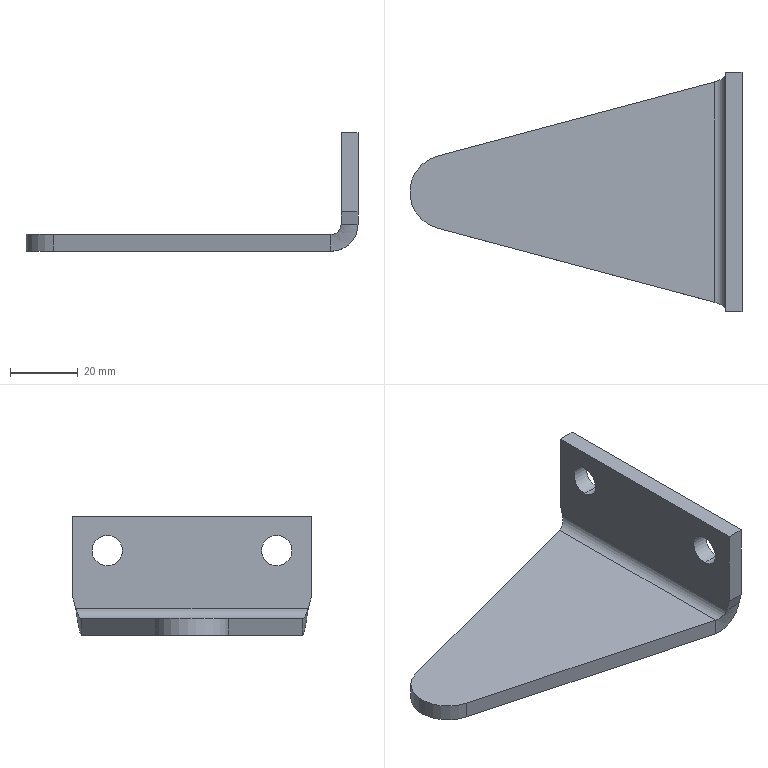Part | SolidWorks | features Fillet 2, BaseBody 1, HoleWzd 1, ICE 1 | 1 solid | 20 faces | box 97.999 x 70.526 x 35.001 mm | volume 30038 mm3 | plane 11 | cylinder 7 | spline 2 | commonest cylinder face diameters 9 x4 6 x1 16 x1 22 x1
STEP:
#1=CARTESIAN_POINT('',(-18.504,39.063,3.138));
#2=VERTEX_POINT('',#1);
#3=CARTESIAN_POINT('',(-18.504,39.063,2.784));
#4=VERTEX_POINT('',#3);
#5=CARTESIAN_POINT('',(-18.504,39.063,2.961));
#6=DIRECTION('',(1.,0.,0.));
#7=DIRECTION('',(0.,1.,0.));
#8=AXIS2_PLACEMENT_3D('',#5,#6,#7);
#9=CIRCLE('',#8,0.1772);
#10=EDGE_CURVE('',#2,#4,#9,.T.);
#11=ORIENTED_EDGE('',*,*,#10,.F.);
#12=CARTESIAN_POINT('',(-18.307,39.063,3.138));
#13=VERTEX_POINT('',#12);
#14=CARTESIAN_POINT('',(-18.307,39.063,3.138));
#15=DIRECTION('',(1.,0.,0.));
#16=VECTOR('',#15,39.37);
#17=LINE('',#14,#16);
#18=EDGE_CURVE('',#2,#13,#17,.T.);
#19=ORIENTED_EDGE('',*,*,#18,.T.);
#20=CARTESIAN_POINT('',(-18.307,39.063,2.784));
#21=VERTEX_POINT('',#20);
#22=CARTESIAN_POINT('',(-18.307,39.063,2.961));
#23=DIRECTION('',(1.,0.,0.));
#24=DIRECTION('',(0.,0.,-1.));
#25=AXIS2_PLACEMENT_3D('',#22,#23,#24);
#26=CIRCLE('',#25,0.1772);
#27=EDGE_CURVE('',#13,#21,#26,.T.);
#28=ORIENTED_EDGE('',*,*,#27,.T.);
#29=CARTESIAN_POINT('',(-18.307,39.063,2.784));
#30=DIRECTION('',(1.,0.,0.));
#31=VECTOR('',#30,39.37);
#32=LINE('',#29,#31);
#33=EDGE_CURVE('',#4,#21,#32,.T.);
#34=ORIENTED_EDGE('',*,*,#33,.F.);
#35=EDGE_LOOP('',(#11,#19,#28,#34));
#36=FACE_OUTER_BOUND('',#35,.T.);
#37=CARTESIAN_POINT('',(-18.307,39.063,2.961));
#38=DIRECTION('',(1.,0.,0.));
#39=DIRECTION('',(0.,0.,-1.));
#40=AXIS2_PLACEMENT_3D('',#37,#38,#39);
#41=CYLINDRICAL_SURFACE('',#40,0.1772);
#42=ADVANCED_FACE('',(#36),#41,.F.);
#43=CARTESIAN_POINT('',(-18.504,37.094,3.138));
#44=VERTEX_POINT('',#43);
#45=CARTESIAN_POINT('',(-18.504,37.094,2.784));
#46=VERTEX_POINT('',#45);
#47=CARTESIAN_POINT('',(-18.504,37.094,2.961));
#48=DIRECTION('',(1.,0.,0.));
#49=DIRECTION('',(0.,1.,0.));
#50=AXIS2_PLACEMENT_3D('',#47,#48,#49);
#51=CIRCLE('',#50,0.1772);
#52=EDGE_CURVE('',#44,#46,#51,.T.);
#53=ORIENTED_EDGE('',*,*,#52,.F.);
#54=CARTESIAN_POINT('',(-18.307,37.094,3.138));
#55=VERTEX_POINT('',#54);
#56=CARTESIAN_POINT('',(-18.307,37.094,3.138));
#57=DIRECTION('',(1.,0.,0.));
#58=VECTOR('',#57,39.37);
#59=LINE('',#56,#58);
#60=EDGE_CURVE('',#44,#55,#59,.T.);
#61=ORIENTED_EDGE('',*,*,#60,.T.);
#62=CARTESIAN_POINT('',(-18.307,37.094,2.784));
#63=VERTEX_POINT('',#62);
#64=CARTESIAN_POINT('',(-18.307,37.094,2.961));
#65=DIRECTION('',(1.,0.,0.));
#66=DIRECTION('',(0.,0.,-1.));
#67=AXIS2_PLACEMENT_3D('',#64,#65,#66);
#68=CIRCLE('',#67,0.1772);
#69=EDGE_CURVE('',#55,#63,#68,.T.);
#70=ORIENTED_EDGE('',*,*,#69,.T.);
#71=CARTESIAN_POINT('',(-18.307,37.094,2.784));
#72=DIRECTION('',(1.,0.,0.));
#73=VECTOR('',#72,39.37);
#74=LINE('',#71,#73);
#75=EDGE_CURVE('',#46,#63,#74,.T.);
#76=ORIENTED_EDGE('',*,*,#75,.F.);
#77=EDGE_LOOP('',(#53,#61,#70,#76));
#78=FACE_OUTER_BOUND('',#77,.T.);
#79=CARTESIAN_POINT('',(-18.307,37.094,2.961));
#80=DIRECTION('',(1.,0.,0.));
#81=DIRECTION('',(0.,0.,-1.));
#82=AXIS2_PLACEMENT_3D('',#79,#80,#81);
#83=CYLINDRICAL_SURFACE('',#82,0.1772);
#84=ADVANCED_FACE('',(#78),#83,.F.);
#85=CARTESIAN_POINT('',(-21.844,38.497,1.976));
#86=VERTEX_POINT('',#85);
#87=CARTESIAN_POINT('',(-18.622,39.358,1.976));
#88=VERTEX_POINT('',#87);
#89=CARTESIAN_POINT('',(-21.844,38.497,1.976));
#90=DIRECTION('',(0.9661,0.2581,0.));
#91=VECTOR('',#90,39.37);
#92=LINE('',#89,#91);
#93=EDGE_CURVE('',#86,#88,#92,.T.);
#94=ORIENTED_EDGE('',*,*,#93,.T.);
#95=CARTESIAN_POINT('',(-18.622,36.8,1.976));
#96=VERTEX_POINT('',#95);
#97=CARTESIAN_POINT('',(-18.622,38.079,1.976));
#98=DIRECTION('',(0.,-1.,0.));
#99=VECTOR('',#98,39.37);
#100=LINE('',#97,#99);
#101=EDGE_CURVE('',#88,#96,#100,.T.);
#102=ORIENTED_EDGE('',*,*,#101,.T.);
#103=CARTESIAN_POINT('',(-21.844,37.66,1.976));
#104=VERTEX_POINT('',#103);
#105=CARTESIAN_POINT('',(-18.622,36.8,1.976));
#106=DIRECTION('',(-0.9661,0.2581,0.));
#107=VECTOR('',#106,39.37);
#108=LINE('',#105,#107);
#109=EDGE_CURVE('',#96,#104,#108,.T.);
#110=ORIENTED_EDGE('',*,*,#109,.T.);
#111=CARTESIAN_POINT('',(-21.732,38.079,1.976));
#112=DIRECTION('',(0.,0.,-1.));
#113=DIRECTION('',(0.,1.,0.));
#114=AXIS2_PLACEMENT_3D('',#111,#112,#113);
#115=CIRCLE('',#114,0.4331);
#116=EDGE_CURVE('',#104,#86,#115,.T.);
#117=ORIENTED_EDGE('',*,*,#116,.T.);
#118=EDGE_LOOP('',(#94,#102,#110,#117));
#119=FACE_OUTER_BOUND('',#118,.T.);
#120=CARTESIAN_POINT('',(-21.732,38.079,1.976));
#121=DIRECTION('',(0.,0.,-1.));
#122=DIRECTION('',(0.,-1.,0.));
#123=AXIS2_PLACEMENT_3D('',#120,#121,#122);
#124=PLANE('',#123);
#125=ADVANCED_FACE('',(#119),#124,.T.);
#126=CARTESIAN_POINT('',(-21.844,38.497,2.173));
#127=VERTEX_POINT('',#126);
#128=CARTESIAN_POINT('',(-21.844,38.497,2.173));
#129=DIRECTION('',(0.,0.,1.));
#130=VECTOR('',#129,39.37);
#131=LINE('',#128,#130);
#132=EDGE_CURVE('',#86,#127,#131,.T.);
#133=ORIENTED_EDGE('',*,*,#132,.T.);
#134=CARTESIAN_POINT('',(-18.622,39.358,2.173));
#135=VERTEX_POINT('',#134);
#136=CARTESIAN_POINT('',(-21.844,38.497,2.173));
#137=DIRECTION('',(0.9661,0.2581,0.));
#138=VECTOR('',#137,39.37);
#139=LINE('',#136,#138);
#140=EDGE_CURVE('',#127,#135,#139,.T.);
#141=ORIENTED_EDGE('',*,*,#140,.T.);
#142=CARTESIAN_POINT('',(-18.622,39.358,2.173));
#143=DIRECTION('',(0.,0.,-1.));
#144=VECTOR('',#143,39.37);
#145=LINE('',#142,#144);
#146=EDGE_CURVE('',#135,#88,#145,.T.);
#147=ORIENTED_EDGE('',*,*,#146,.T.);
#148=ORIENTED_EDGE('',*,*,#93,.F.);
#149=EDGE_LOOP('',(#133,#141,#147,#148));
#150=FACE_OUTER_BOUND('',#149,.T.);
#151=CARTESIAN_POINT('',(-21.844,38.497,2.173));
#152=DIRECTION('',(-0.2581,0.9661,0.));
#153=DIRECTION('',(0.9661,0.2581,0.));
#154=AXIS2_PLACEMENT_3D('',#151,#152,#153);
#155=PLANE('',#154);
#156=ADVANCED_FACE('',(#150),#155,.T.);
#157=CARTESIAN_POINT('',(-21.844,37.66,2.173));
#158=VERTEX_POINT('',#157);
#159=CARTESIAN_POINT('',(-21.732,38.079,2.173));
#160=DIRECTION('',(0.,0.,-1.));
#161=DIRECTION('',(0.,1.,0.));
#162=AXIS2_PLACEMENT_3D('',#159,#160,#161);
#163=CIRCLE('',#162,0.4331);
#164=EDGE_CURVE('',#158,#127,#163,.T.);
#165=ORIENTED_EDGE('',*,*,#164,.T.);
#166=ORIENTED_EDGE('',*,*,#132,.F.);
#167=ORIENTED_EDGE('',*,*,#116,.F.);
#168=CARTESIAN_POINT('',(-21.844,37.66,2.173));
#169=DIRECTION('',(0.,0.,1.));
#170=VECTOR('',#169,39.37);
#171=LINE('',#168,#170);
#172=EDGE_CURVE('',#104,#158,#171,.T.);
#173=ORIENTED_EDGE('',*,*,#172,.T.);
#174=EDGE_LOOP('',(#165,#166,#167,#173));
#175=FACE_OUTER_BOUND('',#174,.T.);
#176=CARTESIAN_POINT('',(-21.732,38.079,2.173));
#177=DIRECTION('',(0.,0.,1.));
#178=DIRECTION('',(0.,1.,0.));
#179=AXIS2_PLACEMENT_3D('',#176,#177,#178);
#180=CYLINDRICAL_SURFACE('',#179,0.4331);
#181=ADVANCED_FACE('',(#175),#180,.T.);
#182=CARTESIAN_POINT('',(-18.622,36.8,2.173));
#183=VERTEX_POINT('',#182);
#184=CARTESIAN_POINT('',(-18.031,36.642,2.173));
#185=DIRECTION('',(-0.9661,0.2581,0.));
#186=VECTOR('',#185,39.37);
#187=LINE('',#184,#186);
#188=EDGE_CURVE('',#183,#158,#187,.T.);
#189=ORIENTED_EDGE('',*,*,#188,.T.);
#190=ORIENTED_EDGE('',*,*,#172,.F.);
#191=ORIENTED_EDGE('',*,*,#109,.F.);
#192=CARTESIAN_POINT('',(-18.622,36.8,2.173));
#193=DIRECTION('',(0.,0.,1.));
#194=VECTOR('',#193,39.37);
#195=LINE('',#192,#194);
#196=EDGE_CURVE('',#96,#183,#195,.T.);
#197=ORIENTED_EDGE('',*,*,#196,.T.);
#198=EDGE_LOOP('',(#189,#190,#191,#197));
#199=FACE_OUTER_BOUND('',#198,.T.);
#200=CARTESIAN_POINT('',(-18.031,36.642,2.173));
#201=DIRECTION('',(-0.2581,-0.9661,0.));
#202=DIRECTION('',(-0.9661,0.2581,0.));
#203=AXIS2_PLACEMENT_3D('',#200,#201,#202);
#204=PLANE('',#203);
#205=ADVANCED_FACE('',(#199),#204,.T.);
#206=ORIENTED_EDGE('',*,*,#188,.F.);
#207=CARTESIAN_POINT('',(-18.622,39.393,2.173));
#208=DIRECTION('',(0.,1.,0.));
#209=VECTOR('',#208,39.37);
#210=LINE('',#207,#209);
#211=EDGE_CURVE('',#183,#135,#210,.T.);
#212=ORIENTED_EDGE('',*,*,#211,.T.);
#213=ORIENTED_EDGE('',*,*,#140,.F.);
#214=ORIENTED_EDGE('',*,*,#164,.F.);
#215=EDGE_LOOP('',(#206,#212,#213,#214));
#216=FACE_OUTER_BOUND('',#215,.T.);
#217=CARTESIAN_POINT('',(-21.732,38.079,2.173));
#218=DIRECTION('',(0.,0.,-1.));
#219=DIRECTION('',(0.,-1.,0.));
#220=AXIS2_PLACEMENT_3D('',#217,#218,#219);
#221=PLANE('',#220);
#222=ADVANCED_FACE('',(#216),#221,.F.);
#223=CARTESIAN_POINT('',(-18.307,39.429,2.291));
#224=VERTEX_POINT('',#223);
#225=CARTESIAN_POINT('',(-18.504,39.429,2.291));
#226=VERTEX_POINT('',#225);
#227=CARTESIAN_POINT('',(-18.406,39.429,2.291));
#228=DIRECTION('',(-1.,0.,0.));
#229=VECTOR('',#228,39.37);
#230=LINE('',#227,#229);
#231=EDGE_CURVE('',#224,#226,#230,.T.);
#232=ORIENTED_EDGE('',*,*,#231,.F.);
#233=CARTESIAN_POINT('',(-18.307,39.429,2.291));
#234=CARTESIAN_POINT('',(-18.307,39.426,2.271));
#235=CARTESIAN_POINT('',(-18.309,39.423,2.25));
#236=CARTESIAN_POINT('',(-18.315,39.419,2.22));
#237=CARTESIAN_POINT('',(-18.318,39.417,2.21));
#238=CARTESIAN_POINT('',(-18.324,39.414,2.19));
#239=CARTESIAN_POINT('',(-18.327,39.413,2.18));
#240=CARTESIAN_POINT('',(-18.339,39.408,2.152));
#241=CARTESIAN_POINT('',(-18.349,39.405,2.134));
#242=CARTESIAN_POINT('',(-18.371,39.399,2.1));
#243=CARTESIAN_POINT('',(-18.385,39.396,2.083));
#244=CARTESIAN_POINT('',(-18.414,39.39,2.054));
#245=CARTESIAN_POINT('',(-18.43,39.388,2.041));
#246=CARTESIAN_POINT('',(-18.455,39.383,2.024));
#247=CARTESIAN_POINT('',(-18.464,39.382,2.019));
#248=CARTESIAN_POINT('',(-18.483,39.379,2.009));
#249=CARTESIAN_POINT('',(-18.492,39.377,2.004));
#250=CARTESIAN_POINT('',(-18.52,39.373,1.993));
#251=CARTESIAN_POINT('',(-18.54,39.37,1.987));
#252=CARTESIAN_POINT('',(-18.581,39.364,1.978));
#253=CARTESIAN_POINT('',(-18.601,39.361,1.976));
#254=CARTESIAN_POINT('',(-18.622,39.358,1.976));
#255=B_SPLINE_CURVE_WITH_KNOTS('',3,(#233,#234,#235,#236,#237,#238,#239,#240,#241,#242,#243,#244,#245,#246,#247,#248,#249,#250,#251,#252,#253,#254),.UNSPECIFIED.,.F.,.F.,(4,2,2,2,2,2,2,2,2,2,4),(0.,0.001578,0.002367,0.003156,0.004734,0.006312,0.00789,0.008679,0.009468,0.01105,0.01262),.UNSPECIFIED.);
#256=EDGE_CURVE('',#224,#88,#255,.T.);
#257=ORIENTED_EDGE('',*,*,#256,.T.);
#258=ORIENTED_EDGE('',*,*,#146,.F.);
#259=CARTESIAN_POINT('',(-18.622,39.358,2.173));
#260=CARTESIAN_POINT('',(-18.614,39.361,2.173));
#261=CARTESIAN_POINT('',(-18.607,39.364,2.174));
#262=CARTESIAN_POINT('',(-18.591,39.37,2.177));
#263=CARTESIAN_POINT('',(-18.584,39.373,2.179));
#264=CARTESIAN_POINT('',(-18.57,39.379,2.185));
#265=CARTESIAN_POINT('',(-18.563,39.382,2.189));
#266=CARTESIAN_POINT('',(-18.55,39.387,2.197));
#267=CARTESIAN_POINT('',(-18.544,39.39,2.202));
#268=CARTESIAN_POINT('',(-18.533,39.396,2.213));
#269=CARTESIAN_POINT('',(-18.528,39.399,2.219));
#270=CARTESIAN_POINT('',(-18.52,39.405,2.232));
#271=CARTESIAN_POINT('',(-18.516,39.408,2.239));
#272=CARTESIAN_POINT('',(-18.51,39.414,2.253));
#273=CARTESIAN_POINT('',(-18.508,39.417,2.261));
#274=CARTESIAN_POINT('',(-18.505,39.423,2.276));
#275=CARTESIAN_POINT('',(-18.504,39.426,2.284));
#276=CARTESIAN_POINT('',(-18.504,39.429,2.291));
#277=B_SPLINE_CURVE_WITH_KNOTS('',3,(#259,#260,#261,#262,#263,#264,#265,#266,#267,#268,#269,#270,#271,#272,#273,#274,#275,#276),.UNSPECIFIED.,.F.,.F.,(4,2,2,2,2,2,2,2,4),(0.,0.0006272,0.001254,0.001881,0.002509,0.003136,0.003763,0.00439,0.005017),.UNSPECIFIED.);
#278=EDGE_CURVE('',#135,#226,#277,.T.);
#279=ORIENTED_EDGE('',*,*,#278,.T.);
#280=EDGE_LOOP('',(#232,#257,#258,#279));
#281=FACE_OUTER_BOUND('',#280,.T.);
#282=CARTESIAN_POINT('',(-18.175,39.429,2.291));
#283=CARTESIAN_POINT('',(-18.175,39.423,2.233));
#284=CARTESIAN_POINT('',(-18.186,39.417,2.174));
#285=CARTESIAN_POINT('',(-18.231,39.405,2.066));
#286=CARTESIAN_POINT('',(-18.264,39.399,2.016));
#287=CARTESIAN_POINT('',(-18.347,39.387,1.934));
#288=CARTESIAN_POINT('',(-18.397,39.382,1.9));
#289=CARTESIAN_POINT('',(-18.505,39.37,1.856));
#290=CARTESIAN_POINT('',(-18.563,39.364,1.844));
#291=CARTESIAN_POINT('',(-18.622,39.358,1.844));
#292=CARTESIAN_POINT('',(-18.305,39.429,2.291));
#293=CARTESIAN_POINT('',(-18.305,39.423,2.25));
#294=CARTESIAN_POINT('',(-18.313,39.417,2.208));
#295=CARTESIAN_POINT('',(-18.345,39.405,2.132));
#296=CARTESIAN_POINT('',(-18.369,39.399,2.097));
#297=CARTESIAN_POINT('',(-18.427,39.387,2.038));
#298=CARTESIAN_POINT('',(-18.462,39.382,2.014));
#299=CARTESIAN_POINT('',(-18.539,39.37,1.983));
#300=CARTESIAN_POINT('',(-18.581,39.364,1.974));
#301=CARTESIAN_POINT('',(-18.622,39.358,1.974));
#302=CARTESIAN_POINT('',(-18.307,39.429,2.291));
#303=CARTESIAN_POINT('',(-18.307,39.423,2.25));
#304=CARTESIAN_POINT('',(-18.315,39.417,2.209));
#305=CARTESIAN_POINT('',(-18.347,39.405,2.133));
#306=CARTESIAN_POINT('',(-18.37,39.399,2.098));
#307=CARTESIAN_POINT('',(-18.428,39.387,2.04));
#308=CARTESIAN_POINT('',(-18.463,39.382,2.016));
#309=CARTESIAN_POINT('',(-18.54,39.37,1.985));
#310=CARTESIAN_POINT('',(-18.581,39.364,1.976));
#311=CARTESIAN_POINT('',(-18.622,39.358,1.976));
#312=CARTESIAN_POINT('',(-18.504,39.429,2.291));
#313=CARTESIAN_POINT('',(-18.504,39.423,2.276));
#314=CARTESIAN_POINT('',(-18.507,39.417,2.26));
#315=CARTESIAN_POINT('',(-18.519,39.405,2.232));
#316=CARTESIAN_POINT('',(-18.528,39.399,2.219));
#317=CARTESIAN_POINT('',(-18.549,39.387,2.197));
#318=CARTESIAN_POINT('',(-18.563,39.382,2.188));
#319=CARTESIAN_POINT('',(-18.591,39.37,2.176));
#320=CARTESIAN_POINT('',(-18.607,39.364,2.173));
#321=CARTESIAN_POINT('',(-18.622,39.358,2.173));
#322=CARTESIAN_POINT('',(-18.506,39.429,2.291));
#323=CARTESIAN_POINT('',(-18.506,39.423,2.276));
#324=CARTESIAN_POINT('',(-18.509,39.417,2.261));
#325=CARTESIAN_POINT('',(-18.521,39.405,2.233));
#326=CARTESIAN_POINT('',(-18.529,39.399,2.22));
#327=CARTESIAN_POINT('',(-18.551,39.387,2.199));
#328=CARTESIAN_POINT('',(-18.564,39.382,2.19));
#329=CARTESIAN_POINT('',(-18.592,39.37,2.178));
#330=CARTESIAN_POINT('',(-18.607,39.364,2.175));
#331=CARTESIAN_POINT('',(-18.622,39.358,2.175));
#332=B_SPLINE_SURFACE_WITH_KNOTS('',1,3,((#282,#283,#284,#285,#286,#287,#288,#289,#290,#291),(#292,#293,#294,#295,#296,#297,#298,#299,#300,#301),(#302,#303,#304,#305,#306,#307,#308,#309,#310,#311),(#312,#313,#314,#315,#316,#317,#318,#319,#320,#321),(#322,#323,#324,#325,#326,#327,#328,#329,#330,#331)),.UNSPECIFIED.,.F.,.F.,.F.,(2,1,1,1,2),(4,2,2,2,4),(-0.6727,-0.01,0.,1.,1.01),(0.,0.25,0.5,0.75,1.),.UNSPECIFIED.);
#333=ADVANCED_FACE('',(#281),#332,.F.);
#334=ORIENTED_EDGE('',*,*,#196,.F.);
#335=CARTESIAN_POINT('',(-18.307,36.729,2.291));
#336=VERTEX_POINT('',#335);
#337=CARTESIAN_POINT('',(-18.622,36.8,1.976));
#338=CARTESIAN_POINT('',(-18.601,36.797,1.976));
#339=CARTESIAN_POINT('',(-18.581,36.794,1.978));
#340=CARTESIAN_POINT('',(-18.551,36.789,1.984));
#341=CARTESIAN_POINT('',(-18.541,36.788,1.987));
#342=CARTESIAN_POINT('',(-18.521,36.785,1.993));
#343=CARTESIAN_POINT('',(-18.511,36.783,1.996));
#344=CARTESIAN_POINT('',(-18.482,36.779,2.008));
#345=CARTESIAN_POINT('',(-18.464,36.776,2.018));
#346=CARTESIAN_POINT('',(-18.43,36.77,2.041));
#347=CARTESIAN_POINT('',(-18.414,36.767,2.054));
#348=CARTESIAN_POINT('',(-18.385,36.761,2.083));
#349=CARTESIAN_POINT('',(-18.372,36.758,2.099));
#350=CARTESIAN_POINT('',(-18.355,36.754,2.125));
#351=CARTESIAN_POINT('',(-18.349,36.752,2.134));
#352=CARTESIAN_POINT('',(-18.339,36.749,2.152));
#353=CARTESIAN_POINT('',(-18.335,36.748,2.161));
#354=CARTESIAN_POINT('',(-18.323,36.743,2.19));
#355=CARTESIAN_POINT('',(-18.317,36.741,2.209));
#356=CARTESIAN_POINT('',(-18.309,36.735,2.25));
#357=CARTESIAN_POINT('',(-18.307,36.732,2.271));
#358=CARTESIAN_POINT('',(-18.307,36.729,2.291));
#359=B_SPLINE_CURVE_WITH_KNOTS('',3,(#337,#338,#339,#340,#341,#342,#343,#344,#345,#346,#347,#348,#349,#350,#351,#352,#353,#354,#355,#356,#357,#358),.UNSPECIFIED.,.F.,.F.,(4,2,2,2,2,2,2,2,2,2,4),(0.,0.001578,0.002367,0.003156,0.004734,0.006312,0.00789,0.008679,0.009468,0.01105,0.01262),.UNSPECIFIED.);
#360=EDGE_CURVE('',#96,#336,#359,.T.);
#361=ORIENTED_EDGE('',*,*,#360,.T.);
#362=CARTESIAN_POINT('',(-18.504,36.729,2.291));
#363=VERTEX_POINT('',#362);
#364=CARTESIAN_POINT('',(-18.406,36.729,2.291));
#365=DIRECTION('',(1.,0.,0.));
#366=VECTOR('',#365,39.37);
#367=LINE('',#364,#366);
#368=EDGE_CURVE('',#363,#336,#367,.T.);
#369=ORIENTED_EDGE('',*,*,#368,.F.);
#370=CARTESIAN_POINT('',(-18.504,36.729,2.291));
#371=CARTESIAN_POINT('',(-18.504,36.732,2.284));
#372=CARTESIAN_POINT('',(-18.505,36.735,2.276));
#373=CARTESIAN_POINT('',(-18.508,36.74,2.261));
#374=CARTESIAN_POINT('',(-18.51,36.743,2.253));
#375=CARTESIAN_POINT('',(-18.516,36.749,2.239));
#376=CARTESIAN_POINT('',(-18.52,36.752,2.232));
#377=CARTESIAN_POINT('',(-18.528,36.758,2.219));
#378=CARTESIAN_POINT('',(-18.533,36.761,2.213));
#379=CARTESIAN_POINT('',(-18.544,36.767,2.202));
#380=CARTESIAN_POINT('',(-18.55,36.77,2.198));
#381=CARTESIAN_POINT('',(-18.563,36.776,2.189));
#382=CARTESIAN_POINT('',(-18.57,36.779,2.185));
#383=CARTESIAN_POINT('',(-18.584,36.785,2.179));
#384=CARTESIAN_POINT('',(-18.591,36.788,2.177));
#385=CARTESIAN_POINT('',(-18.606,36.794,2.174));
#386=CARTESIAN_POINT('',(-18.614,36.797,2.173));
#387=CARTESIAN_POINT('',(-18.622,36.8,2.173));
#388=B_SPLINE_CURVE_WITH_KNOTS('',3,(#370,#371,#372,#373,#374,#375,#376,#377,#378,#379,#380,#381,#382,#383,#384,#385,#386,#387),.UNSPECIFIED.,.F.,.F.,(4,2,2,2,2,2,2,2,4),(0.,0.0006272,0.001254,0.001881,0.002509,0.003136,0.003763,0.00439,0.005017),.UNSPECIFIED.);
#389=EDGE_CURVE('',#363,#183,#388,.T.);
#390=ORIENTED_EDGE('',*,*,#389,.T.);
#391=EDGE_LOOP('',(#334,#361,#369,#390));
#392=FACE_OUTER_BOUND('',#391,.T.);
#393=CARTESIAN_POINT('',(-18.622,36.8,1.844));
#394=CARTESIAN_POINT('',(-18.563,36.794,1.844));
#395=CARTESIAN_POINT('',(-18.505,36.788,1.856));
#396=CARTESIAN_POINT('',(-18.397,36.776,1.9));
#397=CARTESIAN_POINT('',(-18.347,36.77,1.934));
#398=CARTESIAN_POINT('',(-18.264,36.758,2.016));
#399=CARTESIAN_POINT('',(-18.231,36.752,2.066));
#400=CARTESIAN_POINT('',(-18.186,36.74,2.174));
#401=CARTESIAN_POINT('',(-18.175,36.735,2.233));
#402=CARTESIAN_POINT('',(-18.175,36.729,2.291));
#403=CARTESIAN_POINT('',(-18.622,36.8,1.974));
#404=CARTESIAN_POINT('',(-18.581,36.794,1.974));
#405=CARTESIAN_POINT('',(-18.539,36.788,1.983));
#406=CARTESIAN_POINT('',(-18.462,36.776,2.014));
#407=CARTESIAN_POINT('',(-18.427,36.77,2.038));
#408=CARTESIAN_POINT('',(-18.369,36.758,2.097));
#409=CARTESIAN_POINT('',(-18.345,36.752,2.132));
#410=CARTESIAN_POINT('',(-18.313,36.74,2.208));
#411=CARTESIAN_POINT('',(-18.305,36.735,2.25));
#412=CARTESIAN_POINT('',(-18.305,36.729,2.291));
#413=CARTESIAN_POINT('',(-18.622,36.8,1.976));
#414=CARTESIAN_POINT('',(-18.581,36.794,1.976));
#415=CARTESIAN_POINT('',(-18.54,36.788,1.985));
#416=CARTESIAN_POINT('',(-18.463,36.776,2.016));
#417=CARTESIAN_POINT('',(-18.428,36.77,2.04));
#418=CARTESIAN_POINT('',(-18.37,36.758,2.098));
#419=CARTESIAN_POINT('',(-18.347,36.752,2.133));
#420=CARTESIAN_POINT('',(-18.315,36.74,2.209));
#421=CARTESIAN_POINT('',(-18.307,36.735,2.25));
#422=CARTESIAN_POINT('',(-18.307,36.729,2.291));
#423=CARTESIAN_POINT('',(-18.622,36.8,2.173));
#424=CARTESIAN_POINT('',(-18.607,36.794,2.173));
#425=CARTESIAN_POINT('',(-18.591,36.788,2.176));
#426=CARTESIAN_POINT('',(-18.563,36.776,2.188));
#427=CARTESIAN_POINT('',(-18.549,36.77,2.197));
#428=CARTESIAN_POINT('',(-18.528,36.758,2.219));
#429=CARTESIAN_POINT('',(-18.519,36.752,2.232));
#430=CARTESIAN_POINT('',(-18.507,36.74,2.26));
#431=CARTESIAN_POINT('',(-18.504,36.735,2.276));
#432=CARTESIAN_POINT('',(-18.504,36.729,2.291));
#433=CARTESIAN_POINT('',(-18.622,36.8,2.175));
#434=CARTESIAN_POINT('',(-18.607,36.794,2.175));
#435=CARTESIAN_POINT('',(-18.592,36.788,2.178));
#436=CARTESIAN_POINT('',(-18.564,36.776,2.19));
#437=CARTESIAN_POINT('',(-18.551,36.77,2.199));
#438=CARTESIAN_POINT('',(-18.529,36.758,2.22));
#439=CARTESIAN_POINT('',(-18.521,36.752,2.233));
#440=CARTESIAN_POINT('',(-18.509,36.74,2.261));
#441=CARTESIAN_POINT('',(-18.506,36.735,2.276));
#442=CARTESIAN_POINT('',(-18.506,36.729,2.291));
#443=B_SPLINE_SURFACE_WITH_KNOTS('',1,3,((#393,#394,#395,#396,#397,#398,#399,#400,#401,#402),(#403,#404,#405,#406,#407,#408,#409,#410,#411,#412),(#413,#414,#415,#416,#417,#418,#419,#420,#421,#422),(#423,#424,#425,#426,#427,#428,#429,#430,#431,#432),(#433,#434,#435,#436,#437,#438,#439,#440,#441,#442)),.UNSPECIFIED.,.F.,.F.,.F.,(2,1,1,1,2),(4,2,2,2,4),(-0.6727,-0.01,0.,1.,1.01),(0.,0.25,0.5,0.75,1.),.UNSPECIFIED.);
#444=ADVANCED_FACE('',(#392),#443,.F.);
#445=CARTESIAN_POINT('',(-18.307,39.063,2.961));
#446=DIRECTION('',(1.,0.,0.));
#447=DIRECTION('',(0.,0.,-1.));
#448=AXIS2_PLACEMENT_3D('',#445,#446,#447);
#449=CIRCLE('',#448,0.1772);
#450=EDGE_CURVE('',#21,#13,#449,.T.);
#451=ORIENTED_EDGE('',*,*,#450,.F.);
#452=ORIENTED_EDGE('',*,*,#27,.F.);
#453=EDGE_LOOP('',(#451,#452));
#454=FACE_BOUND('',#453,.T.);
#455=CARTESIAN_POINT('',(-18.307,37.094,2.961));
#456=DIRECTION('',(1.,0.,0.));
#457=DIRECTION('',(0.,0.,-1.));
#458=AXIS2_PLACEMENT_3D('',#455,#456,#457);
#459=CIRCLE('',#458,0.1772);
#460=EDGE_CURVE('',#63,#55,#459,.T.);
#461=ORIENTED_EDGE('',*,*,#460,.F.);
#462=ORIENTED_EDGE('',*,*,#69,.F.);
#463=EDGE_LOOP('',(#461,#462));
#464=FACE_BOUND('',#463,.T.);
#465=CARTESIAN_POINT('',(-18.307,36.69,2.434));
#466=VERTEX_POINT('',#465);
#467=CARTESIAN_POINT('',(-18.307,36.726,2.302));
#468=DIRECTION('',(0.,0.2581,-0.9661));
#469=VECTOR('',#468,39.37);
#470=LINE('',#467,#469);
#471=EDGE_CURVE('',#466,#336,#470,.T.);
#472=ORIENTED_EDGE('',*,*,#471,.T.);
#473=CARTESIAN_POINT('',(-18.307,38.079,2.291));
#474=DIRECTION('',(0.,1.,0.));
#475=VECTOR('',#474,39.37);
#476=LINE('',#473,#475);
#477=EDGE_CURVE('',#336,#224,#476,.T.);
#478=ORIENTED_EDGE('',*,*,#477,.T.);
#479=CARTESIAN_POINT('',(-18.307,39.467,2.434));
#480=VERTEX_POINT('',#479);
#481=CARTESIAN_POINT('',(-18.307,39.429,2.291));
#482=DIRECTION('',(0.,0.2581,0.9661));
#483=VECTOR('',#482,39.37);
#484=LINE('',#481,#483);
#485=EDGE_CURVE('',#224,#480,#484,.T.);
#486=ORIENTED_EDGE('',*,*,#485,.T.);
#487=CARTESIAN_POINT('',(-18.307,39.467,3.354));
#488=VERTEX_POINT('',#487);
#489=CARTESIAN_POINT('',(-18.307,39.467,3.354));
#490=DIRECTION('',(0.,0.,-1.));
#491=VECTOR('',#490,39.37);
#492=LINE('',#489,#491);
#493=EDGE_CURVE('',#488,#480,#492,.T.);
#494=ORIENTED_EDGE('',*,*,#493,.F.);
#495=CARTESIAN_POINT('',(-18.307,36.69,3.354));
#496=VERTEX_POINT('',#495);
#497=CARTESIAN_POINT('',(-18.307,39.467,3.354));
#498=DIRECTION('',(0.,1.,0.));
#499=VECTOR('',#498,39.37);
#500=LINE('',#497,#499);
#501=EDGE_CURVE('',#496,#488,#500,.T.);
#502=ORIENTED_EDGE('',*,*,#501,.F.);
#503=CARTESIAN_POINT('',(-18.307,36.69,3.354));
#504=DIRECTION('',(0.,0.,-1.));
#505=VECTOR('',#504,39.37);
#506=LINE('',#503,#505);
#507=EDGE_CURVE('',#496,#466,#506,.T.);
#508=ORIENTED_EDGE('',*,*,#507,.T.);
#509=EDGE_LOOP('',(#472,#478,#486,#494,#502,#508));
#510=FACE_OUTER_BOUND('',#509,.T.);
#511=CARTESIAN_POINT('',(-18.307,38.079,-1.084));
#512=DIRECTION('',(1.,0.,0.));
#513=DIRECTION('',(0.,0.,1.));
#514=AXIS2_PLACEMENT_3D('',#511,#512,#513);
#515=PLANE('',#514);
#516=ADVANCED_FACE('',(#454,#464,#510),#515,.T.);
#517=CARTESIAN_POINT('',(-18.504,39.467,2.434));
#518=VERTEX_POINT('',#517);
#519=CARTESIAN_POINT('',(-18.504,38.497,-1.196));
#520=DIRECTION('',(0.,0.2581,0.9661));
#521=VECTOR('',#520,39.37);
#522=LINE('',#519,#521);
#523=EDGE_CURVE('',#226,#518,#522,.T.);
#524=ORIENTED_EDGE('',*,*,#523,.T.);
#525=CARTESIAN_POINT('',(-18.504,39.467,2.434));
#526=DIRECTION('',(-1.,0.,0.));
#527=VECTOR('',#526,39.37);
#528=LINE('',#525,#527);
#529=EDGE_CURVE('',#480,#518,#528,.T.);
#530=ORIENTED_EDGE('',*,*,#529,.F.);
#531=ORIENTED_EDGE('',*,*,#485,.F.);
#532=ORIENTED_EDGE('',*,*,#231,.T.);
#533=EDGE_LOOP('',(#524,#530,#531,#532));
#534=FACE_OUTER_BOUND('',#533,.T.);
#535=CARTESIAN_POINT('',(-18.504,38.497,-1.196));
#536=DIRECTION('',(0.,0.9661,-0.2581));
#537=DIRECTION('',(0.,-0.2581,-0.9661));
#538=AXIS2_PLACEMENT_3D('',#535,#536,#537);
#539=PLANE('',#538);
#540=ADVANCED_FACE('',(#534),#539,.T.);
#541=ORIENTED_EDGE('',*,*,#471,.F.);
#542=CARTESIAN_POINT('',(-18.504,36.69,2.434));
#543=VERTEX_POINT('',#542);
#544=CARTESIAN_POINT('',(-18.504,36.69,2.434));
#545=DIRECTION('',(1.,0.,0.));
#546=VECTOR('',#545,39.37);
#547=LINE('',#544,#546);
#548=EDGE_CURVE('',#543,#466,#547,.T.);
#549=ORIENTED_EDGE('',*,*,#548,.F.);
#550=CARTESIAN_POINT('',(-18.504,36.642,2.617));
#551=DIRECTION('',(0.,0.2581,-0.9661));
#552=VECTOR('',#551,39.37);
#553=LINE('',#550,#552);
#554=EDGE_CURVE('',#543,#363,#553,.T.);
#555=ORIENTED_EDGE('',*,*,#554,.T.);
#556=ORIENTED_EDGE('',*,*,#368,.T.);
#557=EDGE_LOOP('',(#541,#549,#555,#556));
#558=FACE_OUTER_BOUND('',#557,.T.);
#559=CARTESIAN_POINT('',(-18.504,36.642,2.617));
#560=DIRECTION('',(0.,-0.9661,-0.2581));
#561=DIRECTION('',(0.,-0.2581,0.9661));
#562=AXIS2_PLACEMENT_3D('',#559,#560,#561);
#563=PLANE('',#562);
#564=ADVANCED_FACE('',(#558),#563,.T.);
#565=CARTESIAN_POINT('',(-18.504,39.063,2.961));
#566=DIRECTION('',(1.,0.,0.));
#567=DIRECTION('',(0.,1.,0.));
#568=AXIS2_PLACEMENT_3D('',#565,#566,#567);
#569=CIRCLE('',#568,0.1772);
#570=EDGE_CURVE('',#4,#2,#569,.T.);
#571=ORIENTED_EDGE('',*,*,#570,.T.);
#572=ORIENTED_EDGE('',*,*,#10,.T.);
#573=EDGE_LOOP('',(#571,#572));
#574=FACE_BOUND('',#573,.T.);
#575=CARTESIAN_POINT('',(-18.504,37.094,2.961));
#576=DIRECTION('',(1.,0.,0.));
#577=DIRECTION('',(0.,1.,0.));
#578=AXIS2_PLACEMENT_3D('',#575,#576,#577);
#579=CIRCLE('',#578,0.1772);
#580=EDGE_CURVE('',#46,#44,#579,.T.);
#581=ORIENTED_EDGE('',*,*,#580,.T.);
#582=ORIENTED_EDGE('',*,*,#52,.T.);
#583=EDGE_LOOP('',(#581,#582));
#584=FACE_BOUND('',#583,.T.);
#585=ORIENTED_EDGE('',*,*,#523,.F.);
#586=CARTESIAN_POINT('',(-18.504,36.764,2.291));
#587=DIRECTION('',(0.,-1.,0.));
#588=VECTOR('',#587,39.37);
#589=LINE('',#586,#588);
#590=EDGE_CURVE('',#226,#363,#589,.T.);
#591=ORIENTED_EDGE('',*,*,#590,.T.);
#592=ORIENTED_EDGE('',*,*,#554,.F.);
#593=CARTESIAN_POINT('',(-18.504,36.69,3.354));
#594=VERTEX_POINT('',#593);
#595=CARTESIAN_POINT('',(-18.504,36.69,3.354));
#596=DIRECTION('',(0.,0.,-1.));
#597=VECTOR('',#596,39.37);
#598=LINE('',#595,#597);
#599=EDGE_CURVE('',#594,#543,#598,.T.);
#600=ORIENTED_EDGE('',*,*,#599,.F.);
#601=CARTESIAN_POINT('',(-18.504,39.467,3.354));
#602=VERTEX_POINT('',#601);
#603=CARTESIAN_POINT('',(-18.504,36.69,3.354));
#604=DIRECTION('',(0.,-1.,0.));
#605=VECTOR('',#604,39.37);
#606=LINE('',#603,#605);
#607=EDGE_CURVE('',#602,#594,#606,.T.);
#608=ORIENTED_EDGE('',*,*,#607,.F.);
#609=CARTESIAN_POINT('',(-18.504,39.467,3.354));
#610=DIRECTION('',(0.,0.,-1.));
#611=VECTOR('',#610,39.37);
#612=LINE('',#609,#611);
#613=EDGE_CURVE('',#602,#518,#612,.T.);
#614=ORIENTED_EDGE('',*,*,#613,.T.);
#615=EDGE_LOOP('',(#585,#591,#592,#600,#608,#614));
#616=FACE_OUTER_BOUND('',#615,.T.);
#617=CARTESIAN_POINT('',(-18.504,38.079,-1.084));
#618=DIRECTION('',(1.,0.,0.));
#619=DIRECTION('',(0.,0.,1.));
#620=AXIS2_PLACEMENT_3D('',#617,#618,#619);
#621=PLANE('',#620);
#622=ADVANCED_FACE('',(#574,#584,#616),#621,.F.);
#623=ORIENTED_EDGE('',*,*,#529,.T.);
#624=ORIENTED_EDGE('',*,*,#613,.F.);
#625=CARTESIAN_POINT('',(-18.504,39.467,3.354));
#626=DIRECTION('',(-1.,0.,0.));
#627=VECTOR('',#626,39.37);
#628=LINE('',#625,#627);
#629=EDGE_CURVE('',#488,#602,#628,.T.);
#630=ORIENTED_EDGE('',*,*,#629,.F.);
#631=ORIENTED_EDGE('',*,*,#493,.T.);
#632=EDGE_LOOP('',(#623,#624,#630,#631));
#633=FACE_OUTER_BOUND('',#632,.T.);
#634=CARTESIAN_POINT('',(-18.504,39.467,3.354));
#635=DIRECTION('',(0.,-1.,0.));
#636=DIRECTION('',(0.,0.,-1.));
#637=AXIS2_PLACEMENT_3D('',#634,#635,#636);
#638=PLANE('',#637);
#639=ADVANCED_FACE('',(#633),#638,.F.);
#640=ORIENTED_EDGE('',*,*,#548,.T.);
#641=ORIENTED_EDGE('',*,*,#507,.F.);
#642=CARTESIAN_POINT('',(-18.307,36.69,3.354));
#643=DIRECTION('',(1.,0.,0.));
#644=VECTOR('',#643,39.37);
#645=LINE('',#642,#644);
#646=EDGE_CURVE('',#594,#496,#645,.T.);
#647=ORIENTED_EDGE('',*,*,#646,.F.);
#648=ORIENTED_EDGE('',*,*,#599,.T.);
#649=EDGE_LOOP('',(#640,#641,#647,#648));
#650=FACE_OUTER_BOUND('',#649,.T.);
#651=CARTESIAN_POINT('',(-18.307,36.69,3.354));
#652=DIRECTION('',(0.,1.,0.));
#653=DIRECTION('',(0.,0.,1.));
#654=AXIS2_PLACEMENT_3D('',#651,#652,#653);
#655=PLANE('',#654);
#656=ADVANCED_FACE('',(#650),#655,.F.);
#657=ORIENTED_EDGE('',*,*,#501,.T.);
#658=ORIENTED_EDGE('',*,*,#629,.T.);
#659=ORIENTED_EDGE('',*,*,#607,.T.);
#660=ORIENTED_EDGE('',*,*,#646,.T.);
#661=EDGE_LOOP('',(#657,#658,#659,#660));
#662=FACE_OUTER_BOUND('',#661,.T.);
#663=CARTESIAN_POINT('',(0.,0.,3.354));
#664=DIRECTION('',(0.,0.,-1.));
#665=DIRECTION('',(-1.,0.,0.));
#666=AXIS2_PLACEMENT_3D('',#663,#664,#665);
#667=PLANE('',#666);
#668=ADVANCED_FACE('',(#662),#667,.F.);
#669=ORIENTED_EDGE('',*,*,#60,.F.);
#670=ORIENTED_EDGE('',*,*,#580,.F.);
#671=ORIENTED_EDGE('',*,*,#75,.T.);
#672=ORIENTED_EDGE('',*,*,#460,.T.);
#673=EDGE_LOOP('',(#669,#670,#671,#672));
#674=FACE_OUTER_BOUND('',#673,.T.);
#675=CARTESIAN_POINT('',(-18.307,37.094,2.961));
#676=DIRECTION('',(1.,0.,0.));
#677=DIRECTION('',(0.,0.,-1.));
#678=AXIS2_PLACEMENT_3D('',#675,#676,#677);
#679=CYLINDRICAL_SURFACE('',#678,0.1772);
#680=ADVANCED_FACE('',(#674),#679,.F.);
#681=ORIENTED_EDGE('',*,*,#18,.F.);
#682=ORIENTED_EDGE('',*,*,#570,.F.);
#683=ORIENTED_EDGE('',*,*,#33,.T.);
#684=ORIENTED_EDGE('',*,*,#450,.T.);
#685=EDGE_LOOP('',(#681,#682,#683,#684));
#686=FACE_OUTER_BOUND('',#685,.T.);
#687=CARTESIAN_POINT('',(-18.307,39.063,2.961));
#688=DIRECTION('',(1.,0.,0.));
#689=DIRECTION('',(0.,0.,-1.));
#690=AXIS2_PLACEMENT_3D('',#687,#688,#689);
#691=CYLINDRICAL_SURFACE('',#690,0.1772);
#692=ADVANCED_FACE('',(#686),#691,.F.);
#693=ORIENTED_EDGE('',*,*,#389,.F.);
#694=ORIENTED_EDGE('',*,*,#590,.F.);
#695=ORIENTED_EDGE('',*,*,#278,.F.);
#696=ORIENTED_EDGE('',*,*,#211,.F.);
#697=EDGE_LOOP('',(#693,#694,#695,#696));
#698=FACE_OUTER_BOUND('',#697,.T.);
#699=CARTESIAN_POINT('',(-18.622,38.079,2.291));
#700=DIRECTION('',(0.,-1.,0.));
#701=DIRECTION('',(0.,0.,-1.));
#702=AXIS2_PLACEMENT_3D('',#699,#700,#701);
#703=CYLINDRICAL_SURFACE('',#702,0.1181);
#704=ADVANCED_FACE('',(#698),#703,.F.);
#705=ORIENTED_EDGE('',*,*,#256,.F.);
#706=ORIENTED_EDGE('',*,*,#477,.F.);
#707=ORIENTED_EDGE('',*,*,#360,.F.);
#708=ORIENTED_EDGE('',*,*,#101,.F.);
#709=EDGE_LOOP('',(#705,#706,#707,#708));
#710=FACE_OUTER_BOUND('',#709,.T.);
#711=CARTESIAN_POINT('',(-18.622,38.079,2.291));
#712=DIRECTION('',(0.,-1.,0.));
#713=DIRECTION('',(0.,0.,-1.));
#714=AXIS2_PLACEMENT_3D('',#711,#712,#713);
#715=CYLINDRICAL_SURFACE('',#714,0.315);
#716=ADVANCED_FACE('',(#710),#715,.T.);
#717=CLOSED_SHELL('',(#42,#84,#125,#156,#181,#205,#222,#333,#444,#516,#540,#564,#622,#639,#656,#668,#680,#692,#704,#716));
#718=MANIFOLD_SOLID_BREP('',#717);
#719=CARTESIAN_POINT('',(0.,0.,0.));
#720=DIRECTION('',(0.,0.,1.));
#721=DIRECTION('',(1.,0.,0.));
#722=AXIS2_PLACEMENT_3D('',#719,#720,#721);
#723=(LENGTH_UNIT()NAMED_UNIT(*)SI_UNIT($,.METRE.));
#724=LENGTH_MEASURE_WITH_UNIT(LENGTH_MEASURE(0.0254),#723);
#725=DIMENSIONAL_EXPONENTS(1.,0.,0.,0.,0.,0.,0.);
#726=(CONVERSION_BASED_UNIT('INCH',#724)LENGTH_UNIT()NAMED_UNIT(#725));
#727=UNCERTAINTY_MEASURE_WITH_UNIT(LENGTH_MEASURE(0.00001),#726,'','');
#728=(NAMED_UNIT(*)PLANE_ANGLE_UNIT()SI_UNIT($,.RADIAN.));
#729=(NAMED_UNIT(*)SI_UNIT($,.STERADIAN.)SOLID_ANGLE_UNIT());
#730=(GEOMETRIC_REPRESENTATION_CONTEXT(3)GLOBAL_UNCERTAINTY_ASSIGNED_CONTEXT((#727))GLOBAL_UNIT_ASSIGNED_CONTEXT((#726,#728,#729))REPRESENTATION_CONTEXT('',''));
#731=ADVANCED_BREP_SHAPE_REPRESENTATION('',(#718,#722),#730);